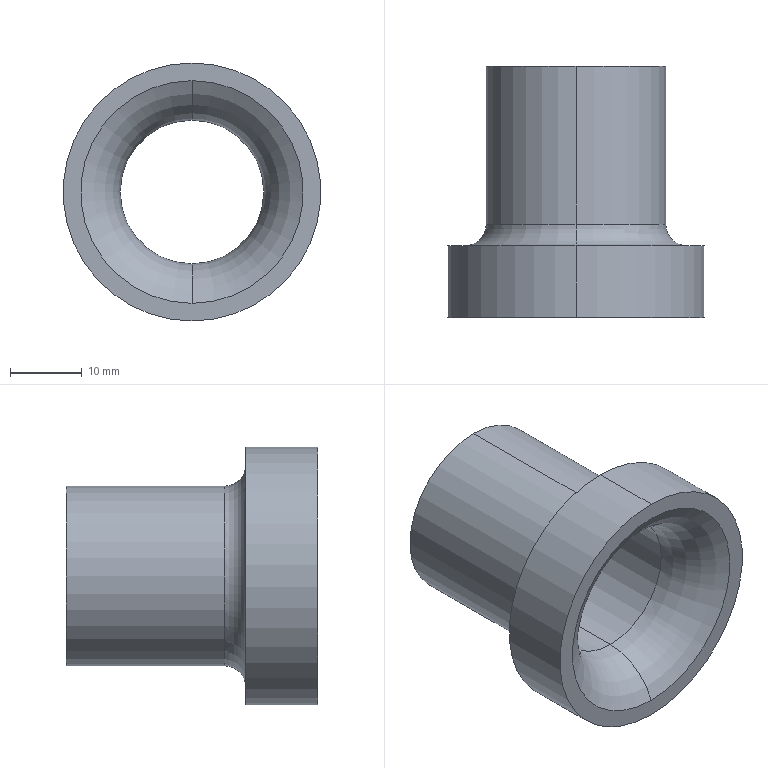Part | SolidWorks | features Revolution 1 | 1 solid | 13 faces | box 35.913 x 35 x 35.913 mm | volume 10695 mm3 | cylinder 6 | torus 4 | plane 3 | commonest cylinder face diameters 20 x2 25 x2 35.913 x2
STEP:
#1=CARTESIAN_POINT('',(0.,6.837,12.5));
#2=VERTEX_POINT('',#1);
#3=CARTESIAN_POINT('',(0.,6.837,-12.5));
#4=VERTEX_POINT('',#3);
#5=CARTESIAN_POINT('',(0.,6.837,0.));
#6=DIRECTION('',(0.,1.,0.));
#7=DIRECTION('',(0.,0.,1.));
#8=AXIS2_PLACEMENT_3D('',#5,#6,#7);
#9=CIRCLE('',#8,12.5);
#10=EDGE_CURVE('',#2,#4,#9,.T.);
#11=ORIENTED_EDGE('',*,*,#10,.T.);
#12=CARTESIAN_POINT('',(0.,28.837,-12.5));
#13=VERTEX_POINT('',#12);
#14=CARTESIAN_POINT('',(0.,10.886,-12.5));
#15=DIRECTION('',(0.,1.,0.));
#16=VECTOR('',#15,1000.);
#17=LINE('',#14,#16);
#18=EDGE_CURVE('',#4,#13,#17,.T.);
#19=ORIENTED_EDGE('',*,*,#18,.T.);
#20=CARTESIAN_POINT('',(0.,28.837,12.5));
#21=VERTEX_POINT('',#20);
#22=CARTESIAN_POINT('',(0.,28.837,0.));
#23=DIRECTION('',(0.,1.,0.));
#24=DIRECTION('',(0.,0.,1.));
#25=AXIS2_PLACEMENT_3D('',#22,#23,#24);
#26=CIRCLE('',#25,12.5);
#27=EDGE_CURVE('',#21,#13,#26,.T.);
#28=ORIENTED_EDGE('',*,*,#27,.F.);
#29=CARTESIAN_POINT('',(0.,10.886,12.5));
#30=DIRECTION('',(0.,1.,0.));
#31=VECTOR('',#30,1000.);
#32=LINE('',#29,#31);
#33=EDGE_CURVE('',#2,#21,#32,.T.);
#34=ORIENTED_EDGE('',*,*,#33,.F.);
#35=EDGE_LOOP('',(#11,#19,#28,#34));
#36=FACE_OUTER_BOUND('',#35,.T.);
#37=CARTESIAN_POINT('',(0.,10.886,0.));
#38=DIRECTION('',(0.,1.,0.));
#39=DIRECTION('',(0.,0.,1.));
#40=AXIS2_PLACEMENT_3D('',#37,#38,#39);
#41=CYLINDRICAL_SURFACE('',#40,12.5);
#42=ADVANCED_FACE('',(#36),#41,.T.);
#43=CARTESIAN_POINT('',(0.,6.837,0.));
#44=DIRECTION('',(0.,1.,0.));
#45=DIRECTION('',(0.,0.,1.));
#46=AXIS2_PLACEMENT_3D('',#43,#44,#45);
#47=CIRCLE('',#46,12.5);
#48=EDGE_CURVE('',#4,#2,#47,.T.);
#49=ORIENTED_EDGE('',*,*,#48,.F.);
#50=CARTESIAN_POINT('',(0.,3.837,-15.5));
#51=VERTEX_POINT('',#50);
#52=CARTESIAN_POINT('',(0.,6.837,-15.5));
#53=DIRECTION('',(1.,0.,0.));
#54=DIRECTION('',(0.,0.,-1.));
#55=AXIS2_PLACEMENT_3D('',#52,#53,#54);
#56=CIRCLE('',#55,3.);
#57=EDGE_CURVE('',#4,#51,#56,.T.);
#58=ORIENTED_EDGE('',*,*,#57,.T.);
#59=CARTESIAN_POINT('',(0.,3.837,15.5));
#60=VERTEX_POINT('',#59);
#61=CARTESIAN_POINT('',(0.,3.837,0.));
#62=DIRECTION('',(0.,1.,0.));
#63=DIRECTION('',(0.,0.,1.));
#64=AXIS2_PLACEMENT_3D('',#61,#62,#63);
#65=CIRCLE('',#64,15.5);
#66=EDGE_CURVE('',#51,#60,#65,.T.);
#67=ORIENTED_EDGE('',*,*,#66,.T.);
#68=CARTESIAN_POINT('',(0.,6.837,15.5));
#69=DIRECTION('',(-1.,0.,0.));
#70=DIRECTION('',(0.,0.,1.));
#71=AXIS2_PLACEMENT_3D('',#68,#69,#70);
#72=CIRCLE('',#71,3.);
#73=EDGE_CURVE('',#2,#60,#72,.T.);
#74=ORIENTED_EDGE('',*,*,#73,.F.);
#75=EDGE_LOOP('',(#49,#58,#67,#74));
#76=FACE_OUTER_BOUND('',#75,.T.);
#77=CARTESIAN_POINT('',(0.,6.837,0.));
#78=DIRECTION('',(0.,1.,0.));
#79=DIRECTION('',(0.,0.,1.));
#80=AXIS2_PLACEMENT_3D('',#77,#78,#79);
#81=TOROIDAL_SURFACE('',#80,15.5,3.);
#82=ADVANCED_FACE('',(#76),#81,.F.);
#83=CARTESIAN_POINT('',(0.,-6.163,17.956));
#84=VERTEX_POINT('',#83);
#85=CARTESIAN_POINT('',(0.,-6.163,-17.956));
#86=VERTEX_POINT('',#85);
#87=CARTESIAN_POINT('',(0.,-6.163,0.));
#88=DIRECTION('',(0.,1.,0.));
#89=DIRECTION('',(0.,0.,1.));
#90=AXIS2_PLACEMENT_3D('',#87,#88,#89);
#91=CIRCLE('',#90,17.956);
#92=EDGE_CURVE('',#84,#86,#91,.T.);
#93=ORIENTED_EDGE('',*,*,#92,.T.);
#94=CARTESIAN_POINT('',(0.,3.837,-17.956));
#95=VERTEX_POINT('',#94);
#96=CARTESIAN_POINT('',(0.,10.886,-17.956));
#97=DIRECTION('',(0.,1.,0.));
#98=VECTOR('',#97,1000.);
#99=LINE('',#96,#98);
#100=EDGE_CURVE('',#86,#95,#99,.T.);
#101=ORIENTED_EDGE('',*,*,#100,.T.);
#102=CARTESIAN_POINT('',(0.,3.837,17.956));
#103=VERTEX_POINT('',#102);
#104=CARTESIAN_POINT('',(0.,3.837,0.));
#105=DIRECTION('',(0.,1.,0.));
#106=DIRECTION('',(0.,0.,1.));
#107=AXIS2_PLACEMENT_3D('',#104,#105,#106);
#108=CIRCLE('',#107,17.956);
#109=EDGE_CURVE('',#103,#95,#108,.T.);
#110=ORIENTED_EDGE('',*,*,#109,.F.);
#111=CARTESIAN_POINT('',(0.,10.886,17.956));
#112=DIRECTION('',(0.,1.,0.));
#113=VECTOR('',#112,1000.);
#114=LINE('',#111,#113);
#115=EDGE_CURVE('',#84,#103,#114,.T.);
#116=ORIENTED_EDGE('',*,*,#115,.F.);
#117=EDGE_LOOP('',(#93,#101,#110,#116));
#118=FACE_OUTER_BOUND('',#117,.T.);
#119=CARTESIAN_POINT('',(0.,10.886,0.));
#120=DIRECTION('',(0.,1.,0.));
#121=DIRECTION('',(0.,0.,1.));
#122=AXIS2_PLACEMENT_3D('',#119,#120,#121);
#123=CYLINDRICAL_SURFACE('',#122,17.956);
#124=ADVANCED_FACE('',(#118),#123,.T.);
#125=CARTESIAN_POINT('',(0.,1.837,10.));
#126=VERTEX_POINT('',#125);
#127=CARTESIAN_POINT('',(0.,1.837,-10.));
#128=VERTEX_POINT('',#127);
#129=CARTESIAN_POINT('',(0.,1.837,0.));
#130=DIRECTION('',(0.,1.,0.));
#131=DIRECTION('',(0.,0.,1.));
#132=AXIS2_PLACEMENT_3D('',#129,#130,#131);
#133=CIRCLE('',#132,10.);
#134=EDGE_CURVE('',#126,#128,#133,.T.);
#135=ORIENTED_EDGE('',*,*,#134,.T.);
#136=CARTESIAN_POINT('',(0.,-6.163,-15.5));
#137=VERTEX_POINT('',#136);
#138=CARTESIAN_POINT('',(0.,1.837,-18.568));
#139=DIRECTION('',(1.,0.,0.));
#140=DIRECTION('',(0.,0.,-1.));
#141=AXIS2_PLACEMENT_3D('',#138,#139,#140);
#142=CIRCLE('',#141,8.568);
#143=EDGE_CURVE('',#128,#137,#142,.T.);
#144=ORIENTED_EDGE('',*,*,#143,.T.);
#145=CARTESIAN_POINT('',(0.,-6.163,15.5));
#146=VERTEX_POINT('',#145);
#147=CARTESIAN_POINT('',(0.,-6.163,0.));
#148=DIRECTION('',(0.,1.,0.));
#149=DIRECTION('',(0.,0.,1.));
#150=AXIS2_PLACEMENT_3D('',#147,#148,#149);
#151=CIRCLE('',#150,15.5);
#152=EDGE_CURVE('',#146,#137,#151,.T.);
#153=ORIENTED_EDGE('',*,*,#152,.F.);
#154=CARTESIAN_POINT('',(0.,1.837,18.568));
#155=DIRECTION('',(-1.,0.,0.));
#156=DIRECTION('',(0.,0.,1.));
#157=AXIS2_PLACEMENT_3D('',#154,#155,#156);
#158=CIRCLE('',#157,8.568);
#159=EDGE_CURVE('',#126,#146,#158,.T.);
#160=ORIENTED_EDGE('',*,*,#159,.F.);
#161=EDGE_LOOP('',(#135,#144,#153,#160));
#162=FACE_OUTER_BOUND('',#161,.T.);
#163=CARTESIAN_POINT('',(0.,1.837,0.));
#164=DIRECTION('',(0.,1.,0.));
#165=DIRECTION('',(0.,0.,1.));
#166=AXIS2_PLACEMENT_3D('',#163,#164,#165);
#167=TOROIDAL_SURFACE('',#166,18.568,8.568);
#168=ADVANCED_FACE('',(#162),#167,.T.);
#169=CARTESIAN_POINT('',(0.,1.837,0.));
#170=DIRECTION('',(0.,1.,0.));
#171=DIRECTION('',(0.,0.,1.));
#172=AXIS2_PLACEMENT_3D('',#169,#170,#171);
#173=CIRCLE('',#172,10.);
#174=EDGE_CURVE('',#128,#126,#173,.T.);
#175=ORIENTED_EDGE('',*,*,#174,.F.);
#176=CARTESIAN_POINT('',(0.,28.837,-10.));
#177=VERTEX_POINT('',#176);
#178=CARTESIAN_POINT('',(0.,10.886,-10.));
#179=DIRECTION('',(0.,1.,0.));
#180=VECTOR('',#179,1000.);
#181=LINE('',#178,#180);
#182=EDGE_CURVE('',#128,#177,#181,.T.);
#183=ORIENTED_EDGE('',*,*,#182,.T.);
#184=CARTESIAN_POINT('',(0.,28.837,10.));
#185=VERTEX_POINT('',#184);
#186=CARTESIAN_POINT('',(0.,28.837,0.));
#187=DIRECTION('',(0.,1.,0.));
#188=DIRECTION('',(0.,0.,1.));
#189=AXIS2_PLACEMENT_3D('',#186,#187,#188);
#190=CIRCLE('',#189,10.);
#191=EDGE_CURVE('',#177,#185,#190,.T.);
#192=ORIENTED_EDGE('',*,*,#191,.T.);
#193=CARTESIAN_POINT('',(0.,10.886,10.));
#194=DIRECTION('',(0.,1.,0.));
#195=VECTOR('',#194,1000.);
#196=LINE('',#193,#195);
#197=EDGE_CURVE('',#126,#185,#196,.T.);
#198=ORIENTED_EDGE('',*,*,#197,.F.);
#199=EDGE_LOOP('',(#175,#183,#192,#198));
#200=FACE_OUTER_BOUND('',#199,.T.);
#201=CARTESIAN_POINT('',(0.,10.886,0.));
#202=DIRECTION('',(0.,1.,0.));
#203=DIRECTION('',(0.,0.,1.));
#204=AXIS2_PLACEMENT_3D('',#201,#202,#203);
#205=CYLINDRICAL_SURFACE('',#204,10.);
#206=ADVANCED_FACE('',(#200),#205,.F.);
#207=ORIENTED_EDGE('',*,*,#182,.F.);
#208=ORIENTED_EDGE('',*,*,#134,.F.);
#209=ORIENTED_EDGE('',*,*,#197,.T.);
#210=CARTESIAN_POINT('',(0.,28.837,0.));
#211=DIRECTION('',(0.,1.,0.));
#212=DIRECTION('',(0.,0.,1.));
#213=AXIS2_PLACEMENT_3D('',#210,#211,#212);
#214=CIRCLE('',#213,10.);
#215=EDGE_CURVE('',#185,#177,#214,.T.);
#216=ORIENTED_EDGE('',*,*,#215,.T.);
#217=EDGE_LOOP('',(#207,#208,#209,#216));
#218=FACE_OUTER_BOUND('',#217,.T.);
#219=CARTESIAN_POINT('',(0.,10.886,0.));
#220=DIRECTION('',(0.,1.,0.));
#221=DIRECTION('',(0.,0.,1.));
#222=AXIS2_PLACEMENT_3D('',#219,#220,#221);
#223=CYLINDRICAL_SURFACE('',#222,10.);
#224=ADVANCED_FACE('',(#218),#223,.F.);
#225=ORIENTED_EDGE('',*,*,#143,.F.);
#226=ORIENTED_EDGE('',*,*,#174,.T.);
#227=ORIENTED_EDGE('',*,*,#159,.T.);
#228=CARTESIAN_POINT('',(0.,-6.163,0.));
#229=DIRECTION('',(0.,1.,0.));
#230=DIRECTION('',(0.,0.,1.));
#231=AXIS2_PLACEMENT_3D('',#228,#229,#230);
#232=CIRCLE('',#231,15.5);
#233=EDGE_CURVE('',#137,#146,#232,.T.);
#234=ORIENTED_EDGE('',*,*,#233,.F.);
#235=EDGE_LOOP('',(#225,#226,#227,#234));
#236=FACE_OUTER_BOUND('',#235,.T.);
#237=CARTESIAN_POINT('',(0.,1.837,0.));
#238=DIRECTION('',(0.,1.,0.));
#239=DIRECTION('',(0.,0.,1.));
#240=AXIS2_PLACEMENT_3D('',#237,#238,#239);
#241=TOROIDAL_SURFACE('',#240,18.568,8.568);
#242=ADVANCED_FACE('',(#236),#241,.T.);
#243=ORIENTED_EDGE('',*,*,#152,.T.);
#244=ORIENTED_EDGE('',*,*,#233,.T.);
#245=EDGE_LOOP('',(#243,#244));
#246=FACE_BOUND('',#245,.T.);
#247=ORIENTED_EDGE('',*,*,#92,.F.);
#248=CARTESIAN_POINT('',(0.,-6.163,0.));
#249=DIRECTION('',(0.,1.,0.));
#250=DIRECTION('',(0.,0.,1.));
#251=AXIS2_PLACEMENT_3D('',#248,#249,#250);
#252=CIRCLE('',#251,17.956);
#253=EDGE_CURVE('',#86,#84,#252,.T.);
#254=ORIENTED_EDGE('',*,*,#253,.F.);
#255=EDGE_LOOP('',(#247,#254));
#256=FACE_OUTER_BOUND('',#255,.T.);
#257=CARTESIAN_POINT('',(-15.5,-6.163,0.));
#258=DIRECTION('',(0.,-1.,0.));
#259=DIRECTION('',(0.,0.,-1.));
#260=AXIS2_PLACEMENT_3D('',#257,#258,#259);
#261=PLANE('',#260);
#262=ADVANCED_FACE('',(#246,#256),#261,.T.);
#263=ORIENTED_EDGE('',*,*,#100,.F.);
#264=ORIENTED_EDGE('',*,*,#253,.T.);
#265=ORIENTED_EDGE('',*,*,#115,.T.);
#266=CARTESIAN_POINT('',(0.,3.837,0.));
#267=DIRECTION('',(0.,1.,0.));
#268=DIRECTION('',(0.,0.,1.));
#269=AXIS2_PLACEMENT_3D('',#266,#267,#268);
#270=CIRCLE('',#269,17.956);
#271=EDGE_CURVE('',#95,#103,#270,.T.);
#272=ORIENTED_EDGE('',*,*,#271,.F.);
#273=EDGE_LOOP('',(#263,#264,#265,#272));
#274=FACE_OUTER_BOUND('',#273,.T.);
#275=CARTESIAN_POINT('',(0.,10.886,0.));
#276=DIRECTION('',(0.,1.,0.));
#277=DIRECTION('',(0.,0.,1.));
#278=AXIS2_PLACEMENT_3D('',#275,#276,#277);
#279=CYLINDRICAL_SURFACE('',#278,17.956);
#280=ADVANCED_FACE('',(#274),#279,.T.);
#281=ORIENTED_EDGE('',*,*,#109,.T.);
#282=ORIENTED_EDGE('',*,*,#271,.T.);
#283=EDGE_LOOP('',(#281,#282));
#284=FACE_OUTER_BOUND('',#283,.T.);
#285=CARTESIAN_POINT('',(0.,3.837,0.));
#286=DIRECTION('',(0.,1.,0.));
#287=DIRECTION('',(0.,0.,1.));
#288=AXIS2_PLACEMENT_3D('',#285,#286,#287);
#289=CIRCLE('',#288,15.5);
#290=EDGE_CURVE('',#60,#51,#289,.T.);
#291=ORIENTED_EDGE('',*,*,#290,.F.);
#292=ORIENTED_EDGE('',*,*,#66,.F.);
#293=EDGE_LOOP('',(#291,#292));
#294=FACE_BOUND('',#293,.T.);
#295=CARTESIAN_POINT('',(-15.5,3.837,0.));
#296=DIRECTION('',(0.,1.,0.));
#297=DIRECTION('',(0.,0.,1.));
#298=AXIS2_PLACEMENT_3D('',#295,#296,#297);
#299=PLANE('',#298);
#300=ADVANCED_FACE('',(#284,#294),#299,.T.);
#301=ORIENTED_EDGE('',*,*,#57,.F.);
#302=ORIENTED_EDGE('',*,*,#10,.F.);
#303=ORIENTED_EDGE('',*,*,#73,.T.);
#304=ORIENTED_EDGE('',*,*,#290,.T.);
#305=EDGE_LOOP('',(#301,#302,#303,#304));
#306=FACE_OUTER_BOUND('',#305,.T.);
#307=CARTESIAN_POINT('',(0.,6.837,0.));
#308=DIRECTION('',(0.,1.,0.));
#309=DIRECTION('',(0.,0.,1.));
#310=AXIS2_PLACEMENT_3D('',#307,#308,#309);
#311=TOROIDAL_SURFACE('',#310,15.5,3.);
#312=ADVANCED_FACE('',(#306),#311,.F.);
#313=ORIENTED_EDGE('',*,*,#18,.F.);
#314=ORIENTED_EDGE('',*,*,#48,.T.);
#315=ORIENTED_EDGE('',*,*,#33,.T.);
#316=CARTESIAN_POINT('',(0.,28.837,0.));
#317=DIRECTION('',(0.,1.,0.));
#318=DIRECTION('',(0.,0.,1.));
#319=AXIS2_PLACEMENT_3D('',#316,#317,#318);
#320=CIRCLE('',#319,12.5);
#321=EDGE_CURVE('',#13,#21,#320,.T.);
#322=ORIENTED_EDGE('',*,*,#321,.F.);
#323=EDGE_LOOP('',(#313,#314,#315,#322));
#324=FACE_OUTER_BOUND('',#323,.T.);
#325=CARTESIAN_POINT('',(0.,10.886,0.));
#326=DIRECTION('',(0.,1.,0.));
#327=DIRECTION('',(0.,0.,1.));
#328=AXIS2_PLACEMENT_3D('',#325,#326,#327);
#329=CYLINDRICAL_SURFACE('',#328,12.5);
#330=ADVANCED_FACE('',(#324),#329,.T.);
#331=ORIENTED_EDGE('',*,*,#27,.T.);
#332=ORIENTED_EDGE('',*,*,#321,.T.);
#333=EDGE_LOOP('',(#331,#332));
#334=FACE_OUTER_BOUND('',#333,.T.);
#335=ORIENTED_EDGE('',*,*,#215,.F.);
#336=ORIENTED_EDGE('',*,*,#191,.F.);
#337=EDGE_LOOP('',(#335,#336));
#338=FACE_BOUND('',#337,.T.);
#339=CARTESIAN_POINT('',(-10.,28.837,0.));
#340=DIRECTION('',(0.,1.,0.));
#341=DIRECTION('',(0.,0.,1.));
#342=AXIS2_PLACEMENT_3D('',#339,#340,#341);
#343=PLANE('',#342);
#344=ADVANCED_FACE('',(#334,#338),#343,.T.);
#345=CLOSED_SHELL('',(#42,#82,#124,#168,#206,#224,#242,#262,#280,#300,#312,#330,#344));
#346=MANIFOLD_SOLID_BREP('',#345);
#347=CARTESIAN_POINT('',(0.,0.,0.));
#348=DIRECTION('',(0.,0.,1.));
#349=DIRECTION('',(1.,0.,0.));
#350=AXIS2_PLACEMENT_3D('',#347,#348,#349);
#351=(LENGTH_UNIT()NAMED_UNIT(*)SI_UNIT(.MILLI.,.METRE.));
#352=UNCERTAINTY_MEASURE_WITH_UNIT(LENGTH_MEASURE(0.00001),#351,'','');
#353=(NAMED_UNIT(*)PLANE_ANGLE_UNIT()SI_UNIT($,.RADIAN.));
#354=(NAMED_UNIT(*)SI_UNIT($,.STERADIAN.)SOLID_ANGLE_UNIT());
#355=(GEOMETRIC_REPRESENTATION_CONTEXT(3)GLOBAL_UNCERTAINTY_ASSIGNED_CONTEXT((#352))GLOBAL_UNIT_ASSIGNED_CONTEXT((#351,#353,#354))REPRESENTATION_CONTEXT('',''));
#356=ADVANCED_BREP_SHAPE_REPRESENTATION('',(#346,#350),#355);